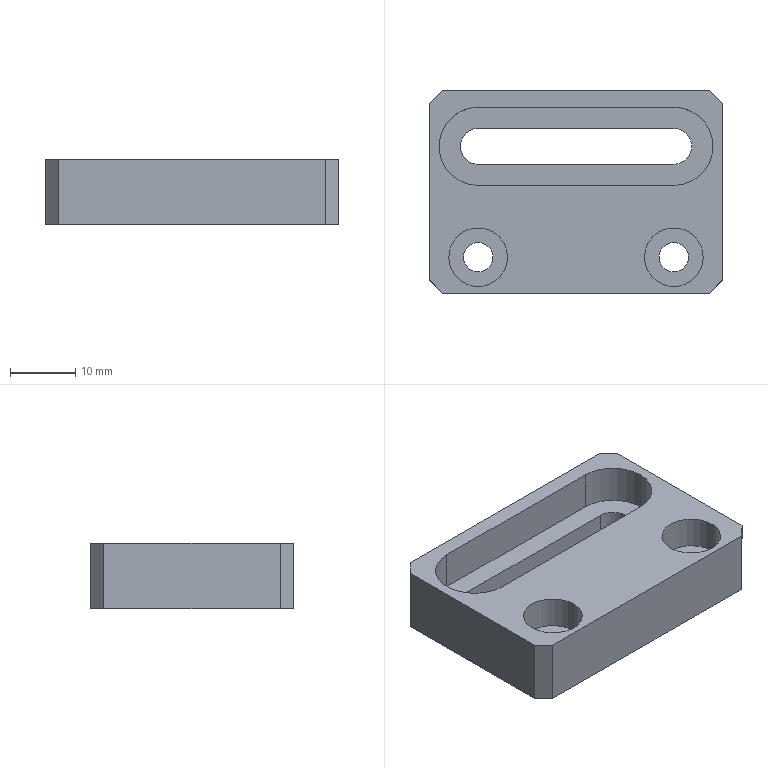Part | SolidWorks | features ICE 4, Chamfer 1, Extrusion 1 | 1 solid | 31 faces | box 45 x 31 x 10 mm | volume 9481 mm3 | plane 17 | cylinder 14 | commonest cylinder face diameters 4.5 x4 9 x4 5.5 x3 12 x3
STEP:
#1=CARTESIAN_POINT('',(21.,7.,4.));
#2=VERTEX_POINT('',#1);
#3=CARTESIAN_POINT('',(15.,13.,4.));
#4=VERTEX_POINT('',#3);
#5=CARTESIAN_POINT('',(15.,7.,4.));
#6=DIRECTION('',(0.,0.,1.));
#7=DIRECTION('',(1.,0.,0.));
#8=AXIS2_PLACEMENT_3D('',#5,#6,#7);
#9=CIRCLE('',#8,6.);
#10=EDGE_CURVE('',#2,#4,#9,.T.);
#11=ORIENTED_EDGE('',*,*,#10,.F.);
#12=CARTESIAN_POINT('',(21.,7.,10.));
#13=VERTEX_POINT('',#12);
#14=CARTESIAN_POINT('',(21.,7.,4.));
#15=DIRECTION('',(0.,0.,1.));
#16=VECTOR('',#15,1000.);
#17=LINE('',#14,#16);
#18=EDGE_CURVE('',#2,#13,#17,.T.);
#19=ORIENTED_EDGE('',*,*,#18,.T.);
#20=CARTESIAN_POINT('',(15.,13.,10.));
#21=VERTEX_POINT('',#20);
#22=CARTESIAN_POINT('',(15.,7.,10.));
#23=DIRECTION('',(0.,0.,1.));
#24=DIRECTION('',(1.,0.,0.));
#25=AXIS2_PLACEMENT_3D('',#22,#23,#24);
#26=CIRCLE('',#25,6.);
#27=EDGE_CURVE('',#13,#21,#26,.T.);
#28=ORIENTED_EDGE('',*,*,#27,.T.);
#29=CARTESIAN_POINT('',(15.,13.,4.));
#30=DIRECTION('',(0.,0.,1.));
#31=VECTOR('',#30,1000.);
#32=LINE('',#29,#31);
#33=EDGE_CURVE('',#4,#21,#32,.T.);
#34=ORIENTED_EDGE('',*,*,#33,.F.);
#35=EDGE_LOOP('',(#11,#19,#28,#34));
#36=FACE_OUTER_BOUND('',#35,.T.);
#37=CARTESIAN_POINT('',(15.,7.,4.));
#38=DIRECTION('',(0.,0.,1.));
#39=DIRECTION('',(1.,0.,0.));
#40=AXIS2_PLACEMENT_3D('',#37,#38,#39);
#41=CYLINDRICAL_SURFACE('',#40,6.);
#42=ADVANCED_FACE('',(#36),#41,.F.);
#43=CARTESIAN_POINT('',(12.75,-10.,0.));
#44=VERTEX_POINT('',#43);
#45=CARTESIAN_POINT('',(17.25,-10.,0.));
#46=VERTEX_POINT('',#45);
#47=CARTESIAN_POINT('',(15.,-10.,0.));
#48=DIRECTION('',(0.,0.,1.));
#49=DIRECTION('',(1.,0.,0.));
#50=AXIS2_PLACEMENT_3D('',#47,#48,#49);
#51=CIRCLE('',#50,2.25);
#52=EDGE_CURVE('',#44,#46,#51,.T.);
#53=ORIENTED_EDGE('',*,*,#52,.F.);
#54=CARTESIAN_POINT('',(12.75,-10.,5.));
#55=VERTEX_POINT('',#54);
#56=CARTESIAN_POINT('',(12.75,-10.,-4.));
#57=DIRECTION('',(0.,0.,1.));
#58=VECTOR('',#57,1000.);
#59=LINE('',#56,#58);
#60=EDGE_CURVE('',#44,#55,#59,.T.);
#61=ORIENTED_EDGE('',*,*,#60,.T.);
#62=CARTESIAN_POINT('',(17.25,-10.,5.));
#63=VERTEX_POINT('',#62);
#64=CARTESIAN_POINT('',(15.,-10.,5.));
#65=DIRECTION('',(0.,0.,-1.));
#66=DIRECTION('',(-1.,0.,0.));
#67=AXIS2_PLACEMENT_3D('',#64,#65,#66);
#68=CIRCLE('',#67,2.25);
#69=EDGE_CURVE('',#63,#55,#68,.T.);
#70=ORIENTED_EDGE('',*,*,#69,.F.);
#71=CARTESIAN_POINT('',(17.25,-10.,-4.));
#72=DIRECTION('',(0.,0.,1.));
#73=VECTOR('',#72,1000.);
#74=LINE('',#71,#73);
#75=EDGE_CURVE('',#46,#63,#74,.T.);
#76=ORIENTED_EDGE('',*,*,#75,.F.);
#77=EDGE_LOOP('',(#53,#61,#70,#76));
#78=FACE_OUTER_BOUND('',#77,.T.);
#79=CARTESIAN_POINT('',(15.,-10.,-4.));
#80=DIRECTION('',(0.,0.,1.));
#81=DIRECTION('',(1.,0.,0.));
#82=AXIS2_PLACEMENT_3D('',#79,#80,#81);
#83=CYLINDRICAL_SURFACE('',#82,2.25);
#84=ADVANCED_FACE('',(#78),#83,.F.);
#85=CARTESIAN_POINT('',(-17.25,-10.,0.));
#86=VERTEX_POINT('',#85);
#87=CARTESIAN_POINT('',(-12.75,-10.,0.));
#88=VERTEX_POINT('',#87);
#89=CARTESIAN_POINT('',(-15.,-10.,0.));
#90=DIRECTION('',(0.,0.,1.));
#91=DIRECTION('',(1.,0.,0.));
#92=AXIS2_PLACEMENT_3D('',#89,#90,#91);
#93=CIRCLE('',#92,2.25);
#94=EDGE_CURVE('',#86,#88,#93,.T.);
#95=ORIENTED_EDGE('',*,*,#94,.F.);
#96=CARTESIAN_POINT('',(-17.25,-10.,5.));
#97=VERTEX_POINT('',#96);
#98=CARTESIAN_POINT('',(-17.25,-10.,-4.));
#99=DIRECTION('',(0.,0.,1.));
#100=VECTOR('',#99,1000.);
#101=LINE('',#98,#100);
#102=EDGE_CURVE('',#86,#97,#101,.T.);
#103=ORIENTED_EDGE('',*,*,#102,.T.);
#104=CARTESIAN_POINT('',(-12.75,-10.,5.));
#105=VERTEX_POINT('',#104);
#106=CARTESIAN_POINT('',(-15.,-10.,5.));
#107=DIRECTION('',(0.,0.,1.));
#108=DIRECTION('',(1.,0.,0.));
#109=AXIS2_PLACEMENT_3D('',#106,#107,#108);
#110=CIRCLE('',#109,2.25);
#111=EDGE_CURVE('',#97,#105,#110,.T.);
#112=ORIENTED_EDGE('',*,*,#111,.T.);
#113=CARTESIAN_POINT('',(-12.75,-10.,-4.));
#114=DIRECTION('',(0.,0.,1.));
#115=VECTOR('',#114,1000.);
#116=LINE('',#113,#115);
#117=EDGE_CURVE('',#88,#105,#116,.T.);
#118=ORIENTED_EDGE('',*,*,#117,.F.);
#119=EDGE_LOOP('',(#95,#103,#112,#118));
#120=FACE_OUTER_BOUND('',#119,.T.);
#121=CARTESIAN_POINT('',(-15.,-10.,-4.));
#122=DIRECTION('',(0.,0.,1.));
#123=DIRECTION('',(1.,0.,0.));
#124=AXIS2_PLACEMENT_3D('',#121,#122,#123);
#125=CYLINDRICAL_SURFACE('',#124,2.25);
#126=ADVANCED_FACE('',(#120),#125,.F.);
#127=CARTESIAN_POINT('',(10.5,-10.,5.));
#128=VERTEX_POINT('',#127);
#129=CARTESIAN_POINT('',(19.5,-10.,5.));
#130=VERTEX_POINT('',#129);
#131=CARTESIAN_POINT('',(15.,-10.,5.));
#132=DIRECTION('',(0.,0.,1.));
#133=DIRECTION('',(-1.,0.,0.));
#134=AXIS2_PLACEMENT_3D('',#131,#132,#133);
#135=CIRCLE('',#134,4.5);
#136=EDGE_CURVE('',#128,#130,#135,.T.);
#137=ORIENTED_EDGE('',*,*,#136,.F.);
#138=CARTESIAN_POINT('',(10.5,-10.,10.));
#139=VERTEX_POINT('',#138);
#140=CARTESIAN_POINT('',(10.5,-10.,5.));
#141=DIRECTION('',(0.,0.,1.));
#142=VECTOR('',#141,1000.);
#143=LINE('',#140,#142);
#144=EDGE_CURVE('',#128,#139,#143,.T.);
#145=ORIENTED_EDGE('',*,*,#144,.T.);
#146=CARTESIAN_POINT('',(19.5,-10.,10.));
#147=VERTEX_POINT('',#146);
#148=CARTESIAN_POINT('',(15.,-10.,10.));
#149=DIRECTION('',(0.,0.,1.));
#150=DIRECTION('',(-1.,0.,0.));
#151=AXIS2_PLACEMENT_3D('',#148,#149,#150);
#152=CIRCLE('',#151,4.5);
#153=EDGE_CURVE('',#139,#147,#152,.T.);
#154=ORIENTED_EDGE('',*,*,#153,.T.);
#155=CARTESIAN_POINT('',(19.5,-10.,5.));
#156=DIRECTION('',(0.,0.,1.));
#157=VECTOR('',#156,1000.);
#158=LINE('',#155,#157);
#159=EDGE_CURVE('',#130,#147,#158,.T.);
#160=ORIENTED_EDGE('',*,*,#159,.F.);
#161=EDGE_LOOP('',(#137,#145,#154,#160));
#162=FACE_OUTER_BOUND('',#161,.T.);
#163=CARTESIAN_POINT('',(15.,-10.,5.));
#164=DIRECTION('',(0.,0.,1.));
#165=DIRECTION('',(1.,0.,0.));
#166=AXIS2_PLACEMENT_3D('',#163,#164,#165);
#167=CYLINDRICAL_SURFACE('',#166,4.5);
#168=ADVANCED_FACE('',(#162),#167,.F.);
#169=CARTESIAN_POINT('',(-19.5,-10.,5.));
#170=VERTEX_POINT('',#169);
#171=CARTESIAN_POINT('',(-10.5,-10.,5.));
#172=VERTEX_POINT('',#171);
#173=CARTESIAN_POINT('',(-15.,-10.,5.));
#174=DIRECTION('',(0.,0.,1.));
#175=DIRECTION('',(1.,0.,0.));
#176=AXIS2_PLACEMENT_3D('',#173,#174,#175);
#177=CIRCLE('',#176,4.5);
#178=EDGE_CURVE('',#170,#172,#177,.T.);
#179=ORIENTED_EDGE('',*,*,#178,.F.);
#180=CARTESIAN_POINT('',(-19.5,-10.,10.));
#181=VERTEX_POINT('',#180);
#182=CARTESIAN_POINT('',(-19.5,-10.,5.));
#183=DIRECTION('',(0.,0.,1.));
#184=VECTOR('',#183,1000.);
#185=LINE('',#182,#184);
#186=EDGE_CURVE('',#170,#181,#185,.T.);
#187=ORIENTED_EDGE('',*,*,#186,.T.);
#188=CARTESIAN_POINT('',(-10.5,-10.,10.));
#189=VERTEX_POINT('',#188);
#190=CARTESIAN_POINT('',(-15.,-10.,10.));
#191=DIRECTION('',(0.,0.,1.));
#192=DIRECTION('',(1.,0.,0.));
#193=AXIS2_PLACEMENT_3D('',#190,#191,#192);
#194=CIRCLE('',#193,4.5);
#195=EDGE_CURVE('',#181,#189,#194,.T.);
#196=ORIENTED_EDGE('',*,*,#195,.T.);
#197=CARTESIAN_POINT('',(-10.5,-10.,5.));
#198=DIRECTION('',(0.,0.,1.));
#199=VECTOR('',#198,1000.);
#200=LINE('',#197,#199);
#201=EDGE_CURVE('',#172,#189,#200,.T.);
#202=ORIENTED_EDGE('',*,*,#201,.F.);
#203=EDGE_LOOP('',(#179,#187,#196,#202));
#204=FACE_OUTER_BOUND('',#203,.T.);
#205=CARTESIAN_POINT('',(-15.,-10.,5.));
#206=DIRECTION('',(0.,0.,1.));
#207=DIRECTION('',(1.,0.,0.));
#208=AXIS2_PLACEMENT_3D('',#205,#206,#207);
#209=CYLINDRICAL_SURFACE('',#208,4.5);
#210=ADVANCED_FACE('',(#204),#209,.F.);
#211=CARTESIAN_POINT('',(17.75,7.,0.));
#212=VERTEX_POINT('',#211);
#213=CARTESIAN_POINT('',(15.,9.75,0.));
#214=VERTEX_POINT('',#213);
#215=CARTESIAN_POINT('',(15.,7.,0.));
#216=DIRECTION('',(0.,0.,1.));
#217=DIRECTION('',(1.,0.,0.));
#218=AXIS2_PLACEMENT_3D('',#215,#216,#217);
#219=CIRCLE('',#218,2.75);
#220=EDGE_CURVE('',#212,#214,#219,.T.);
#221=ORIENTED_EDGE('',*,*,#220,.F.);
#222=CARTESIAN_POINT('',(17.75,7.,4.));
#223=VERTEX_POINT('',#222);
#224=CARTESIAN_POINT('',(17.75,7.,-3.));
#225=DIRECTION('',(0.,0.,1.));
#226=VECTOR('',#225,1000.);
#227=LINE('',#224,#226);
#228=EDGE_CURVE('',#212,#223,#227,.T.);
#229=ORIENTED_EDGE('',*,*,#228,.T.);
#230=CARTESIAN_POINT('',(15.,9.75,4.));
#231=VERTEX_POINT('',#230);
#232=CARTESIAN_POINT('',(15.,7.,4.));
#233=DIRECTION('',(0.,0.,-1.));
#234=DIRECTION('',(1.,0.,0.));
#235=AXIS2_PLACEMENT_3D('',#232,#233,#234);
#236=CIRCLE('',#235,2.75);
#237=EDGE_CURVE('',#231,#223,#236,.T.);
#238=ORIENTED_EDGE('',*,*,#237,.F.);
#239=CARTESIAN_POINT('',(15.,9.75,-3.));
#240=DIRECTION('',(0.,0.,1.));
#241=VECTOR('',#240,1000.);
#242=LINE('',#239,#241);
#243=EDGE_CURVE('',#214,#231,#242,.T.);
#244=ORIENTED_EDGE('',*,*,#243,.F.);
#245=EDGE_LOOP('',(#221,#229,#238,#244));
#246=FACE_OUTER_BOUND('',#245,.T.);
#247=CARTESIAN_POINT('',(15.,7.,-3.));
#248=DIRECTION('',(0.,0.,1.));
#249=DIRECTION('',(1.,0.,0.));
#250=AXIS2_PLACEMENT_3D('',#247,#248,#249);
#251=CYLINDRICAL_SURFACE('',#250,2.75);
#252=ADVANCED_FACE('',(#246),#251,.F.);
#253=CARTESIAN_POINT('',(-15.,4.25,4.));
#254=VERTEX_POINT('',#253);
#255=CARTESIAN_POINT('',(-15.,9.75,4.));
#256=VERTEX_POINT('',#255);
#257=CARTESIAN_POINT('',(-15.,7.,4.));
#258=DIRECTION('',(0.,0.,-1.));
#259=DIRECTION('',(1.,0.,0.));
#260=AXIS2_PLACEMENT_3D('',#257,#258,#259);
#261=CIRCLE('',#260,2.75);
#262=EDGE_CURVE('',#254,#256,#261,.T.);
#263=ORIENTED_EDGE('',*,*,#262,.F.);
#264=CARTESIAN_POINT('',(-15.,4.25,0.));
#265=VERTEX_POINT('',#264);
#266=CARTESIAN_POINT('',(-15.,4.25,-3.));
#267=DIRECTION('',(0.,0.,1.));
#268=VECTOR('',#267,1000.);
#269=LINE('',#266,#268);
#270=EDGE_CURVE('',#265,#254,#269,.T.);
#271=ORIENTED_EDGE('',*,*,#270,.F.);
#272=CARTESIAN_POINT('',(-15.,9.75,0.));
#273=VERTEX_POINT('',#272);
#274=CARTESIAN_POINT('',(-15.,7.,0.));
#275=DIRECTION('',(0.,0.,1.));
#276=DIRECTION('',(1.,0.,0.));
#277=AXIS2_PLACEMENT_3D('',#274,#275,#276);
#278=CIRCLE('',#277,2.75);
#279=EDGE_CURVE('',#273,#265,#278,.T.);
#280=ORIENTED_EDGE('',*,*,#279,.F.);
#281=CARTESIAN_POINT('',(-15.,9.75,-3.));
#282=DIRECTION('',(0.,0.,1.));
#283=VECTOR('',#282,1000.);
#284=LINE('',#281,#283);
#285=EDGE_CURVE('',#273,#256,#284,.T.);
#286=ORIENTED_EDGE('',*,*,#285,.T.);
#287=EDGE_LOOP('',(#263,#271,#280,#286));
#288=FACE_OUTER_BOUND('',#287,.T.);
#289=CARTESIAN_POINT('',(-15.,7.,-3.));
#290=DIRECTION('',(0.,0.,1.));
#291=DIRECTION('',(1.,0.,0.));
#292=AXIS2_PLACEMENT_3D('',#289,#290,#291);
#293=CYLINDRICAL_SURFACE('',#292,2.75);
#294=ADVANCED_FACE('',(#288),#293,.F.);
#295=CARTESIAN_POINT('',(-15.,9.75,4.));
#296=DIRECTION('',(1.,0.,0.));
#297=VECTOR('',#296,1000.);
#298=LINE('',#295,#297);
#299=EDGE_CURVE('',#256,#231,#298,.T.);
#300=ORIENTED_EDGE('',*,*,#299,.F.);
#301=ORIENTED_EDGE('',*,*,#285,.F.);
#302=CARTESIAN_POINT('',(0.,9.75,0.));
#303=DIRECTION('',(-1.,0.,0.));
#304=VECTOR('',#303,1000.);
#305=LINE('',#302,#304);
#306=EDGE_CURVE('',#214,#273,#305,.T.);
#307=ORIENTED_EDGE('',*,*,#306,.F.);
#308=ORIENTED_EDGE('',*,*,#243,.T.);
#309=EDGE_LOOP('',(#300,#301,#307,#308));
#310=FACE_OUTER_BOUND('',#309,.T.);
#311=CARTESIAN_POINT('',(-15.,9.75,-3.));
#312=DIRECTION('',(0.,1.,0.));
#313=DIRECTION('',(-1.,0.,0.));
#314=AXIS2_PLACEMENT_3D('',#311,#312,#313);
#315=PLANE('',#314);
#316=ADVANCED_FACE('',(#310),#315,.F.);
#317=ORIENTED_EDGE('',*,*,#228,.F.);
#318=CARTESIAN_POINT('',(15.,4.25,0.));
#319=VERTEX_POINT('',#318);
#320=CARTESIAN_POINT('',(15.,7.,0.));
#321=DIRECTION('',(0.,0.,1.));
#322=DIRECTION('',(1.,0.,0.));
#323=AXIS2_PLACEMENT_3D('',#320,#321,#322);
#324=CIRCLE('',#323,2.75);
#325=EDGE_CURVE('',#319,#212,#324,.T.);
#326=ORIENTED_EDGE('',*,*,#325,.F.);
#327=CARTESIAN_POINT('',(15.,4.25,4.));
#328=VERTEX_POINT('',#327);
#329=CARTESIAN_POINT('',(15.,4.25,-3.));
#330=DIRECTION('',(0.,0.,1.));
#331=VECTOR('',#330,1000.);
#332=LINE('',#329,#331);
#333=EDGE_CURVE('',#319,#328,#332,.T.);
#334=ORIENTED_EDGE('',*,*,#333,.T.);
#335=CARTESIAN_POINT('',(15.,7.,4.));
#336=DIRECTION('',(0.,0.,-1.));
#337=DIRECTION('',(1.,0.,0.));
#338=AXIS2_PLACEMENT_3D('',#335,#336,#337);
#339=CIRCLE('',#338,2.75);
#340=EDGE_CURVE('',#223,#328,#339,.T.);
#341=ORIENTED_EDGE('',*,*,#340,.F.);
#342=EDGE_LOOP('',(#317,#326,#334,#341));
#343=FACE_OUTER_BOUND('',#342,.T.);
#344=CARTESIAN_POINT('',(15.,7.,-3.));
#345=DIRECTION('',(0.,0.,1.));
#346=DIRECTION('',(1.,0.,0.));
#347=AXIS2_PLACEMENT_3D('',#344,#345,#346);
#348=CYLINDRICAL_SURFACE('',#347,2.75);
#349=ADVANCED_FACE('',(#343),#348,.F.);
#350=CARTESIAN_POINT('',(-15.,4.25,4.));
#351=DIRECTION('',(-1.,0.,0.));
#352=VECTOR('',#351,1000.);
#353=LINE('',#350,#352);
#354=EDGE_CURVE('',#328,#254,#353,.T.);
#355=ORIENTED_EDGE('',*,*,#354,.F.);
#356=ORIENTED_EDGE('',*,*,#333,.F.);
#357=CARTESIAN_POINT('',(0.,4.25,0.));
#358=DIRECTION('',(1.,0.,0.));
#359=VECTOR('',#358,1000.);
#360=LINE('',#357,#359);
#361=EDGE_CURVE('',#265,#319,#360,.T.);
#362=ORIENTED_EDGE('',*,*,#361,.F.);
#363=ORIENTED_EDGE('',*,*,#270,.T.);
#364=EDGE_LOOP('',(#355,#356,#362,#363));
#365=FACE_OUTER_BOUND('',#364,.T.);
#366=CARTESIAN_POINT('',(-15.,4.25,-3.));
#367=DIRECTION('',(0.,-1.,0.));
#368=DIRECTION('',(0.,0.,-1.));
#369=AXIS2_PLACEMENT_3D('',#366,#367,#368);
#370=PLANE('',#369);
#371=ADVANCED_FACE('',(#365),#370,.F.);
#372=CARTESIAN_POINT('',(22.5,-13.5,0.));
#373=VERTEX_POINT('',#372);
#374=CARTESIAN_POINT('',(22.5,13.5,0.));
#375=VERTEX_POINT('',#374);
#376=CARTESIAN_POINT('',(22.5,15.5,0.));
#377=DIRECTION('',(0.,1.,0.));
#378=VECTOR('',#377,1000.);
#379=LINE('',#376,#378);
#380=EDGE_CURVE('',#373,#375,#379,.T.);
#381=ORIENTED_EDGE('',*,*,#380,.T.);
#382=CARTESIAN_POINT('',(22.5,13.5,10.));
#383=VERTEX_POINT('',#382);
#384=CARTESIAN_POINT('',(22.5,13.5,10.));
#385=DIRECTION('',(0.,0.,1.));
#386=VECTOR('',#385,1000.);
#387=LINE('',#384,#386);
#388=EDGE_CURVE('',#375,#383,#387,.T.);
#389=ORIENTED_EDGE('',*,*,#388,.T.);
#390=CARTESIAN_POINT('',(22.5,-13.5,10.));
#391=VERTEX_POINT('',#390);
#392=CARTESIAN_POINT('',(22.5,15.5,10.));
#393=DIRECTION('',(0.,1.,0.));
#394=VECTOR('',#393,1000.);
#395=LINE('',#392,#394);
#396=EDGE_CURVE('',#391,#383,#395,.T.);
#397=ORIENTED_EDGE('',*,*,#396,.F.);
#398=CARTESIAN_POINT('',(22.5,-13.5,10.));
#399=DIRECTION('',(0.,0.,-1.));
#400=VECTOR('',#399,1000.);
#401=LINE('',#398,#400);
#402=EDGE_CURVE('',#391,#373,#401,.T.);
#403=ORIENTED_EDGE('',*,*,#402,.T.);
#404=EDGE_LOOP('',(#381,#389,#397,#403));
#405=FACE_OUTER_BOUND('',#404,.T.);
#406=CARTESIAN_POINT('',(22.5,15.5,10.));
#407=DIRECTION('',(-1.,0.,0.));
#408=DIRECTION('',(0.,-1.,0.));
#409=AXIS2_PLACEMENT_3D('',#406,#407,#408);
#410=PLANE('',#409);
#411=ADVANCED_FACE('',(#405),#410,.F.);
#412=CARTESIAN_POINT('',(20.5,15.5,10.));
#413=VERTEX_POINT('',#412);
#414=CARTESIAN_POINT('',(-20.5,15.5,10.));
#415=VERTEX_POINT('',#414);
#416=CARTESIAN_POINT('',(-22.5,15.5,10.));
#417=DIRECTION('',(-1.,0.,0.));
#418=VECTOR('',#417,1000.);
#419=LINE('',#416,#418);
#420=EDGE_CURVE('',#413,#415,#419,.T.);
#421=ORIENTED_EDGE('',*,*,#420,.F.);
#422=CARTESIAN_POINT('',(20.5,15.5,0.));
#423=VERTEX_POINT('',#422);
#424=CARTESIAN_POINT('',(20.5,15.5,10.));
#425=DIRECTION('',(0.,0.,-1.));
#426=VECTOR('',#425,1000.);
#427=LINE('',#424,#426);
#428=EDGE_CURVE('',#413,#423,#427,.T.);
#429=ORIENTED_EDGE('',*,*,#428,.T.);
#430=CARTESIAN_POINT('',(-20.5,15.5,0.));
#431=VERTEX_POINT('',#430);
#432=CARTESIAN_POINT('',(-22.5,15.5,0.));
#433=DIRECTION('',(-1.,0.,0.));
#434=VECTOR('',#433,1000.);
#435=LINE('',#432,#434);
#436=EDGE_CURVE('',#423,#431,#435,.T.);
#437=ORIENTED_EDGE('',*,*,#436,.T.);
#438=CARTESIAN_POINT('',(-20.5,15.5,10.));
#439=DIRECTION('',(0.,0.,1.));
#440=VECTOR('',#439,1000.);
#441=LINE('',#438,#440);
#442=EDGE_CURVE('',#431,#415,#441,.T.);
#443=ORIENTED_EDGE('',*,*,#442,.T.);
#444=EDGE_LOOP('',(#421,#429,#437,#443));
#445=FACE_OUTER_BOUND('',#444,.T.);
#446=CARTESIAN_POINT('',(-22.5,15.5,10.));
#447=DIRECTION('',(0.,-1.,0.));
#448=DIRECTION('',(0.,0.,-1.));
#449=AXIS2_PLACEMENT_3D('',#446,#447,#448);
#450=PLANE('',#449);
#451=ADVANCED_FACE('',(#445),#450,.F.);
#452=CARTESIAN_POINT('',(-22.5,13.5,0.));
#453=VERTEX_POINT('',#452);
#454=CARTESIAN_POINT('',(-22.5,-13.5,0.));
#455=VERTEX_POINT('',#454);
#456=CARTESIAN_POINT('',(-22.5,15.5,0.));
#457=DIRECTION('',(0.,-1.,0.));
#458=VECTOR('',#457,1000.);
#459=LINE('',#456,#458);
#460=EDGE_CURVE('',#453,#455,#459,.T.);
#461=ORIENTED_EDGE('',*,*,#460,.T.);
#462=CARTESIAN_POINT('',(-22.5,-13.5,10.));
#463=VERTEX_POINT('',#462);
#464=CARTESIAN_POINT('',(-22.5,-13.5,10.));
#465=DIRECTION('',(0.,0.,1.));
#466=VECTOR('',#465,1000.);
#467=LINE('',#464,#466);
#468=EDGE_CURVE('',#455,#463,#467,.T.);
#469=ORIENTED_EDGE('',*,*,#468,.T.);
#470=CARTESIAN_POINT('',(-22.5,13.5,10.));
#471=VERTEX_POINT('',#470);
#472=CARTESIAN_POINT('',(-22.5,15.5,10.));
#473=DIRECTION('',(0.,-1.,0.));
#474=VECTOR('',#473,1000.);
#475=LINE('',#472,#474);
#476=EDGE_CURVE('',#471,#463,#475,.T.);
#477=ORIENTED_EDGE('',*,*,#476,.F.);
#478=CARTESIAN_POINT('',(-22.5,13.5,10.));
#479=DIRECTION('',(0.,0.,-1.));
#480=VECTOR('',#479,1000.);
#481=LINE('',#478,#480);
#482=EDGE_CURVE('',#471,#453,#481,.T.);
#483=ORIENTED_EDGE('',*,*,#482,.T.);
#484=EDGE_LOOP('',(#461,#469,#477,#483));
#485=FACE_OUTER_BOUND('',#484,.T.);
#486=CARTESIAN_POINT('',(-22.5,15.5,10.));
#487=DIRECTION('',(1.,0.,0.));
#488=DIRECTION('',(0.,1.,0.));
#489=AXIS2_PLACEMENT_3D('',#486,#487,#488);
#490=PLANE('',#489);
#491=ADVANCED_FACE('',(#485),#490,.F.);
#492=CARTESIAN_POINT('',(-20.5,-15.5,0.));
#493=VERTEX_POINT('',#492);
#494=CARTESIAN_POINT('',(20.5,-15.5,0.));
#495=VERTEX_POINT('',#494);
#496=CARTESIAN_POINT('',(-22.5,-15.5,0.));
#497=DIRECTION('',(1.,0.,0.));
#498=VECTOR('',#497,1000.);
#499=LINE('',#496,#498);
#500=EDGE_CURVE('',#493,#495,#499,.T.);
#501=ORIENTED_EDGE('',*,*,#500,.T.);
#502=CARTESIAN_POINT('',(20.5,-15.5,10.));
#503=VERTEX_POINT('',#502);
#504=CARTESIAN_POINT('',(20.5,-15.5,10.));
#505=DIRECTION('',(0.,0.,1.));
#506=VECTOR('',#505,1000.);
#507=LINE('',#504,#506);
#508=EDGE_CURVE('',#495,#503,#507,.T.);
#509=ORIENTED_EDGE('',*,*,#508,.T.);
#510=CARTESIAN_POINT('',(-20.5,-15.5,10.));
#511=VERTEX_POINT('',#510);
#512=CARTESIAN_POINT('',(-22.5,-15.5,10.));
#513=DIRECTION('',(1.,0.,0.));
#514=VECTOR('',#513,1000.);
#515=LINE('',#512,#514);
#516=EDGE_CURVE('',#511,#503,#515,.T.);
#517=ORIENTED_EDGE('',*,*,#516,.F.);
#518=CARTESIAN_POINT('',(-20.5,-15.5,10.));
#519=DIRECTION('',(0.,0.,-1.));
#520=VECTOR('',#519,1000.);
#521=LINE('',#518,#520);
#522=EDGE_CURVE('',#511,#493,#521,.T.);
#523=ORIENTED_EDGE('',*,*,#522,.T.);
#524=EDGE_LOOP('',(#501,#509,#517,#523));
#525=FACE_OUTER_BOUND('',#524,.T.);
#526=CARTESIAN_POINT('',(-22.5,-15.5,10.));
#527=DIRECTION('',(0.,1.,0.));
#528=DIRECTION('',(0.,0.,1.));
#529=AXIS2_PLACEMENT_3D('',#526,#527,#528);
#530=PLANE('',#529);
#531=ADVANCED_FACE('',(#525),#530,.F.);
#532=CARTESIAN_POINT('',(-15.,13.,10.));
#533=VERTEX_POINT('',#532);
#534=CARTESIAN_POINT('',(-15.,1.,10.));
#535=VERTEX_POINT('',#534);
#536=CARTESIAN_POINT('',(-15.,7.,10.));
#537=DIRECTION('',(0.,0.,1.));
#538=DIRECTION('',(1.,0.,0.));
#539=AXIS2_PLACEMENT_3D('',#536,#537,#538);
#540=CIRCLE('',#539,6.);
#541=EDGE_CURVE('',#533,#535,#540,.T.);
#542=ORIENTED_EDGE('',*,*,#541,.F.);
#543=CARTESIAN_POINT('',(-15.,13.,10.));
#544=DIRECTION('',(-1.,0.,0.));
#545=VECTOR('',#544,1000.);
#546=LINE('',#543,#545);
#547=EDGE_CURVE('',#21,#533,#546,.T.);
#548=ORIENTED_EDGE('',*,*,#547,.F.);
#549=ORIENTED_EDGE('',*,*,#27,.F.);
#550=CARTESIAN_POINT('',(15.,1.,10.));
#551=VERTEX_POINT('',#550);
#552=CARTESIAN_POINT('',(15.,7.,10.));
#553=DIRECTION('',(0.,0.,1.));
#554=DIRECTION('',(1.,0.,0.));
#555=AXIS2_PLACEMENT_3D('',#552,#553,#554);
#556=CIRCLE('',#555,6.);
#557=EDGE_CURVE('',#551,#13,#556,.T.);
#558=ORIENTED_EDGE('',*,*,#557,.F.);
#559=CARTESIAN_POINT('',(-15.,1.,10.));
#560=DIRECTION('',(1.,0.,0.));
#561=VECTOR('',#560,1000.);
#562=LINE('',#559,#561);
#563=EDGE_CURVE('',#535,#551,#562,.T.);
#564=ORIENTED_EDGE('',*,*,#563,.F.);
#565=EDGE_LOOP('',(#542,#548,#549,#558,#564));
#566=FACE_BOUND('',#565,.T.);
#567=CARTESIAN_POINT('',(15.,-10.,10.));
#568=DIRECTION('',(0.,0.,1.));
#569=DIRECTION('',(-1.,0.,0.));
#570=AXIS2_PLACEMENT_3D('',#567,#568,#569);
#571=CIRCLE('',#570,4.5);
#572=EDGE_CURVE('',#147,#139,#571,.T.);
#573=ORIENTED_EDGE('',*,*,#572,.F.);
#574=ORIENTED_EDGE('',*,*,#153,.F.);
#575=EDGE_LOOP('',(#573,#574));
#576=FACE_BOUND('',#575,.T.);
#577=CARTESIAN_POINT('',(-15.,-10.,10.));
#578=DIRECTION('',(0.,0.,1.));
#579=DIRECTION('',(1.,0.,0.));
#580=AXIS2_PLACEMENT_3D('',#577,#578,#579);
#581=CIRCLE('',#580,4.5);
#582=EDGE_CURVE('',#189,#181,#581,.T.);
#583=ORIENTED_EDGE('',*,*,#582,.F.);
#584=ORIENTED_EDGE('',*,*,#195,.F.);
#585=EDGE_LOOP('',(#583,#584));
#586=FACE_BOUND('',#585,.T.);
#587=ORIENTED_EDGE('',*,*,#396,.T.);
#588=CARTESIAN_POINT('',(18.,18.,10.));
#589=DIRECTION('',(-0.7071,0.7071,0.));
#590=VECTOR('',#589,1000.);
#591=LINE('',#588,#590);
#592=EDGE_CURVE('',#383,#413,#591,.T.);
#593=ORIENTED_EDGE('',*,*,#592,.T.);
#594=ORIENTED_EDGE('',*,*,#420,.T.);
#595=CARTESIAN_POINT('',(-18.,18.,10.));
#596=DIRECTION('',(-0.7071,-0.7071,0.));
#597=VECTOR('',#596,1000.);
#598=LINE('',#595,#597);
#599=EDGE_CURVE('',#415,#471,#598,.T.);
#600=ORIENTED_EDGE('',*,*,#599,.T.);
#601=ORIENTED_EDGE('',*,*,#476,.T.);
#602=CARTESIAN_POINT('',(-18.,-18.,10.));
#603=DIRECTION('',(0.7071,-0.7071,0.));
#604=VECTOR('',#603,1000.);
#605=LINE('',#602,#604);
#606=EDGE_CURVE('',#463,#511,#605,.T.);
#607=ORIENTED_EDGE('',*,*,#606,.T.);
#608=ORIENTED_EDGE('',*,*,#516,.T.);
#609=CARTESIAN_POINT('',(18.,-18.,10.));
#610=DIRECTION('',(0.7071,0.7071,0.));
#611=VECTOR('',#610,1000.);
#612=LINE('',#609,#611);
#613=EDGE_CURVE('',#503,#391,#612,.T.);
#614=ORIENTED_EDGE('',*,*,#613,.T.);
#615=EDGE_LOOP('',(#587,#593,#594,#600,#601,#607,#608,#614));
#616=FACE_OUTER_BOUND('',#615,.T.);
#617=CARTESIAN_POINT('',(0.,0.,10.));
#618=DIRECTION('',(0.,0.,1.));
#619=DIRECTION('',(1.,0.,0.));
#620=AXIS2_PLACEMENT_3D('',#617,#618,#619);
#621=PLANE('',#620);
#622=ADVANCED_FACE('',(#566,#576,#586,#616),#621,.T.);
#623=CARTESIAN_POINT('',(15.,-10.,0.));
#624=DIRECTION('',(0.,0.,1.));
#625=DIRECTION('',(1.,0.,0.));
#626=AXIS2_PLACEMENT_3D('',#623,#624,#625);
#627=CIRCLE('',#626,2.25);
#628=EDGE_CURVE('',#46,#44,#627,.T.);
#629=ORIENTED_EDGE('',*,*,#628,.T.);
#630=ORIENTED_EDGE('',*,*,#52,.T.);
#631=EDGE_LOOP('',(#629,#630));
#632=FACE_BOUND('',#631,.T.);
#633=CARTESIAN_POINT('',(-15.,-10.,0.));
#634=DIRECTION('',(0.,0.,1.));
#635=DIRECTION('',(1.,0.,0.));
#636=AXIS2_PLACEMENT_3D('',#633,#634,#635);
#637=CIRCLE('',#636,2.25);
#638=EDGE_CURVE('',#88,#86,#637,.T.);
#639=ORIENTED_EDGE('',*,*,#638,.T.);
#640=ORIENTED_EDGE('',*,*,#94,.T.);
#641=EDGE_LOOP('',(#639,#640));
#642=FACE_BOUND('',#641,.T.);
#643=ORIENTED_EDGE('',*,*,#306,.T.);
#644=ORIENTED_EDGE('',*,*,#279,.T.);
#645=ORIENTED_EDGE('',*,*,#361,.T.);
#646=ORIENTED_EDGE('',*,*,#325,.T.);
#647=ORIENTED_EDGE('',*,*,#220,.T.);
#648=EDGE_LOOP('',(#643,#644,#645,#646,#647));
#649=FACE_BOUND('',#648,.T.);
#650=ORIENTED_EDGE('',*,*,#436,.F.);
#651=CARTESIAN_POINT('',(20.5,15.5,0.));
#652=DIRECTION('',(0.7071,-0.7071,0.));
#653=VECTOR('',#652,1000.);
#654=LINE('',#651,#653);
#655=EDGE_CURVE('',#423,#375,#654,.T.);
#656=ORIENTED_EDGE('',*,*,#655,.T.);
#657=ORIENTED_EDGE('',*,*,#380,.F.);
#658=CARTESIAN_POINT('',(22.5,-13.5,0.));
#659=DIRECTION('',(-0.7071,-0.7071,0.));
#660=VECTOR('',#659,1000.);
#661=LINE('',#658,#660);
#662=EDGE_CURVE('',#373,#495,#661,.T.);
#663=ORIENTED_EDGE('',*,*,#662,.T.);
#664=ORIENTED_EDGE('',*,*,#500,.F.);
#665=CARTESIAN_POINT('',(-20.5,-15.5,0.));
#666=DIRECTION('',(-0.7071,0.7071,0.));
#667=VECTOR('',#666,1000.);
#668=LINE('',#665,#667);
#669=EDGE_CURVE('',#493,#455,#668,.T.);
#670=ORIENTED_EDGE('',*,*,#669,.T.);
#671=ORIENTED_EDGE('',*,*,#460,.F.);
#672=CARTESIAN_POINT('',(-22.5,13.5,0.));
#673=DIRECTION('',(0.7071,0.7071,0.));
#674=VECTOR('',#673,1000.);
#675=LINE('',#672,#674);
#676=EDGE_CURVE('',#453,#431,#675,.T.);
#677=ORIENTED_EDGE('',*,*,#676,.T.);
#678=EDGE_LOOP('',(#650,#656,#657,#663,#664,#670,#671,#677));
#679=FACE_OUTER_BOUND('',#678,.T.);
#680=CARTESIAN_POINT('',(0.,0.,0.));
#681=DIRECTION('',(0.,0.,1.));
#682=DIRECTION('',(1.,0.,0.));
#683=AXIS2_PLACEMENT_3D('',#680,#681,#682);
#684=PLANE('',#683);
#685=ADVANCED_FACE('',(#632,#642,#649,#679),#684,.F.);
#686=ORIENTED_EDGE('',*,*,#186,.F.);
#687=CARTESIAN_POINT('',(-15.,-10.,5.));
#688=DIRECTION('',(0.,0.,1.));
#689=DIRECTION('',(1.,0.,0.));
#690=AXIS2_PLACEMENT_3D('',#687,#688,#689);
#691=CIRCLE('',#690,4.5);
#692=EDGE_CURVE('',#172,#170,#691,.T.);
#693=ORIENTED_EDGE('',*,*,#692,.F.);
#694=ORIENTED_EDGE('',*,*,#201,.T.);
#695=ORIENTED_EDGE('',*,*,#582,.T.);
#696=EDGE_LOOP('',(#686,#693,#694,#695));
#697=FACE_OUTER_BOUND('',#696,.T.);
#698=CARTESIAN_POINT('',(-15.,-10.,5.));
#699=DIRECTION('',(0.,0.,1.));
#700=DIRECTION('',(1.,0.,0.));
#701=AXIS2_PLACEMENT_3D('',#698,#699,#700);
#702=CYLINDRICAL_SURFACE('',#701,4.5);
#703=ADVANCED_FACE('',(#697),#702,.F.);
#704=CARTESIAN_POINT('',(-15.,-10.,5.));
#705=DIRECTION('',(0.,0.,1.));
#706=DIRECTION('',(1.,0.,0.));
#707=AXIS2_PLACEMENT_3D('',#704,#705,#706);
#708=CIRCLE('',#707,2.25);
#709=EDGE_CURVE('',#105,#97,#708,.T.);
#710=ORIENTED_EDGE('',*,*,#709,.F.);
#711=ORIENTED_EDGE('',*,*,#111,.F.);
#712=EDGE_LOOP('',(#710,#711));
#713=FACE_BOUND('',#712,.T.);
#714=ORIENTED_EDGE('',*,*,#692,.T.);
#715=ORIENTED_EDGE('',*,*,#178,.T.);
#716=EDGE_LOOP('',(#714,#715));
#717=FACE_OUTER_BOUND('',#716,.T.);
#718=CARTESIAN_POINT('',(-15.,-10.,5.));
#719=DIRECTION('',(0.,0.,1.));
#720=DIRECTION('',(1.,0.,0.));
#721=AXIS2_PLACEMENT_3D('',#718,#719,#720);
#722=PLANE('',#721);
#723=ADVANCED_FACE('',(#713,#717),#722,.T.);
#724=ORIENTED_EDGE('',*,*,#144,.F.);
#725=CARTESIAN_POINT('',(15.,-10.,5.));
#726=DIRECTION('',(0.,0.,1.));
#727=DIRECTION('',(-1.,0.,0.));
#728=AXIS2_PLACEMENT_3D('',#725,#726,#727);
#729=CIRCLE('',#728,4.5);
#730=EDGE_CURVE('',#130,#128,#729,.T.);
#731=ORIENTED_EDGE('',*,*,#730,.F.);
#732=ORIENTED_EDGE('',*,*,#159,.T.);
#733=ORIENTED_EDGE('',*,*,#572,.T.);
#734=EDGE_LOOP('',(#724,#731,#732,#733));
#735=FACE_OUTER_BOUND('',#734,.T.);
#736=CARTESIAN_POINT('',(15.,-10.,5.));
#737=DIRECTION('',(0.,0.,1.));
#738=DIRECTION('',(1.,0.,0.));
#739=AXIS2_PLACEMENT_3D('',#736,#737,#738);
#740=CYLINDRICAL_SURFACE('',#739,4.5);
#741=ADVANCED_FACE('',(#735),#740,.F.);
#742=ORIENTED_EDGE('',*,*,#69,.T.);
#743=CARTESIAN_POINT('',(15.,-10.,5.));
#744=DIRECTION('',(0.,0.,-1.));
#745=DIRECTION('',(-1.,0.,0.));
#746=AXIS2_PLACEMENT_3D('',#743,#744,#745);
#747=CIRCLE('',#746,2.25);
#748=EDGE_CURVE('',#55,#63,#747,.T.);
#749=ORIENTED_EDGE('',*,*,#748,.T.);
#750=EDGE_LOOP('',(#742,#749));
#751=FACE_BOUND('',#750,.T.);
#752=ORIENTED_EDGE('',*,*,#730,.T.);
#753=ORIENTED_EDGE('',*,*,#136,.T.);
#754=EDGE_LOOP('',(#752,#753));
#755=FACE_OUTER_BOUND('',#754,.T.);
#756=CARTESIAN_POINT('',(15.,-10.,5.));
#757=DIRECTION('',(0.,0.,-1.));
#758=DIRECTION('',(-1.,0.,0.));
#759=AXIS2_PLACEMENT_3D('',#756,#757,#758);
#760=PLANE('',#759);
#761=ADVANCED_FACE('',(#751,#755),#760,.F.);
#762=ORIENTED_EDGE('',*,*,#102,.F.);
#763=ORIENTED_EDGE('',*,*,#638,.F.);
#764=ORIENTED_EDGE('',*,*,#117,.T.);
#765=ORIENTED_EDGE('',*,*,#709,.T.);
#766=EDGE_LOOP('',(#762,#763,#764,#765));
#767=FACE_OUTER_BOUND('',#766,.T.);
#768=CARTESIAN_POINT('',(-15.,-10.,-4.));
#769=DIRECTION('',(0.,0.,1.));
#770=DIRECTION('',(1.,0.,0.));
#771=AXIS2_PLACEMENT_3D('',#768,#769,#770);
#772=CYLINDRICAL_SURFACE('',#771,2.25);
#773=ADVANCED_FACE('',(#767),#772,.F.);
#774=ORIENTED_EDGE('',*,*,#60,.F.);
#775=ORIENTED_EDGE('',*,*,#628,.F.);
#776=ORIENTED_EDGE('',*,*,#75,.T.);
#777=ORIENTED_EDGE('',*,*,#748,.F.);
#778=EDGE_LOOP('',(#774,#775,#776,#777));
#779=FACE_OUTER_BOUND('',#778,.T.);
#780=CARTESIAN_POINT('',(15.,-10.,-4.));
#781=DIRECTION('',(0.,0.,1.));
#782=DIRECTION('',(1.,0.,0.));
#783=AXIS2_PLACEMENT_3D('',#780,#781,#782);
#784=CYLINDRICAL_SURFACE('',#783,2.25);
#785=ADVANCED_FACE('',(#779),#784,.F.);
#786=ORIENTED_EDGE('',*,*,#592,.F.);
#787=ORIENTED_EDGE('',*,*,#388,.F.);
#788=ORIENTED_EDGE('',*,*,#655,.F.);
#789=ORIENTED_EDGE('',*,*,#428,.F.);
#790=EDGE_LOOP('',(#786,#787,#788,#789));
#791=FACE_OUTER_BOUND('',#790,.T.);
#792=CARTESIAN_POINT('',(20.5,15.5,10.));
#793=DIRECTION('',(-0.7071,-0.7071,0.));
#794=DIRECTION('',(0.,0.,-1.));
#795=AXIS2_PLACEMENT_3D('',#792,#793,#794);
#796=PLANE('',#795);
#797=ADVANCED_FACE('',(#791),#796,.F.);
#798=ORIENTED_EDGE('',*,*,#613,.F.);
#799=ORIENTED_EDGE('',*,*,#508,.F.);
#800=ORIENTED_EDGE('',*,*,#662,.F.);
#801=ORIENTED_EDGE('',*,*,#402,.F.);
#802=EDGE_LOOP('',(#798,#799,#800,#801));
#803=FACE_OUTER_BOUND('',#802,.T.);
#804=CARTESIAN_POINT('',(22.5,-13.5,10.));
#805=DIRECTION('',(-0.7071,0.7071,0.));
#806=DIRECTION('',(0.,0.,-1.));
#807=AXIS2_PLACEMENT_3D('',#804,#805,#806);
#808=PLANE('',#807);
#809=ADVANCED_FACE('',(#803),#808,.F.);
#810=ORIENTED_EDGE('',*,*,#606,.F.);
#811=ORIENTED_EDGE('',*,*,#468,.F.);
#812=ORIENTED_EDGE('',*,*,#669,.F.);
#813=ORIENTED_EDGE('',*,*,#522,.F.);
#814=EDGE_LOOP('',(#810,#811,#812,#813));
#815=FACE_OUTER_BOUND('',#814,.T.);
#816=CARTESIAN_POINT('',(-20.5,-15.5,10.));
#817=DIRECTION('',(0.7071,0.7071,0.));
#818=DIRECTION('',(0.,0.,-1.));
#819=AXIS2_PLACEMENT_3D('',#816,#817,#818);
#820=PLANE('',#819);
#821=ADVANCED_FACE('',(#815),#820,.F.);
#822=ORIENTED_EDGE('',*,*,#599,.F.);
#823=ORIENTED_EDGE('',*,*,#442,.F.);
#824=ORIENTED_EDGE('',*,*,#676,.F.);
#825=ORIENTED_EDGE('',*,*,#482,.F.);
#826=EDGE_LOOP('',(#822,#823,#824,#825));
#827=FACE_OUTER_BOUND('',#826,.T.);
#828=CARTESIAN_POINT('',(-22.5,13.5,10.));
#829=DIRECTION('',(0.7071,-0.7071,0.));
#830=DIRECTION('',(0.,0.,-1.));
#831=AXIS2_PLACEMENT_3D('',#828,#829,#830);
#832=PLANE('',#831);
#833=ADVANCED_FACE('',(#827),#832,.F.);
#834=CARTESIAN_POINT('',(-15.,13.,4.));
#835=VERTEX_POINT('',#834);
#836=CARTESIAN_POINT('',(-15.,1.,4.));
#837=VERTEX_POINT('',#836);
#838=CARTESIAN_POINT('',(-15.,7.,4.));
#839=DIRECTION('',(0.,0.,1.));
#840=DIRECTION('',(1.,0.,0.));
#841=AXIS2_PLACEMENT_3D('',#838,#839,#840);
#842=CIRCLE('',#841,6.);
#843=EDGE_CURVE('',#835,#837,#842,.T.);
#844=ORIENTED_EDGE('',*,*,#843,.T.);
#845=CARTESIAN_POINT('',(15.,1.,4.));
#846=VERTEX_POINT('',#845);
#847=CARTESIAN_POINT('',(-15.,1.,4.));
#848=DIRECTION('',(1.,0.,0.));
#849=VECTOR('',#848,1000.);
#850=LINE('',#847,#849);
#851=EDGE_CURVE('',#837,#846,#850,.T.);
#852=ORIENTED_EDGE('',*,*,#851,.T.);
#853=CARTESIAN_POINT('',(15.,7.,4.));
#854=DIRECTION('',(0.,0.,1.));
#855=DIRECTION('',(1.,0.,0.));
#856=AXIS2_PLACEMENT_3D('',#853,#854,#855);
#857=CIRCLE('',#856,6.);
#858=EDGE_CURVE('',#846,#2,#857,.T.);
#859=ORIENTED_EDGE('',*,*,#858,.T.);
#860=ORIENTED_EDGE('',*,*,#10,.T.);
#861=CARTESIAN_POINT('',(-15.,13.,4.));
#862=DIRECTION('',(-1.,0.,0.));
#863=VECTOR('',#862,1000.);
#864=LINE('',#861,#863);
#865=EDGE_CURVE('',#4,#835,#864,.T.);
#866=ORIENTED_EDGE('',*,*,#865,.T.);
#867=EDGE_LOOP('',(#844,#852,#859,#860,#866));
#868=FACE_OUTER_BOUND('',#867,.T.);
#869=ORIENTED_EDGE('',*,*,#262,.T.);
#870=ORIENTED_EDGE('',*,*,#299,.T.);
#871=ORIENTED_EDGE('',*,*,#237,.T.);
#872=ORIENTED_EDGE('',*,*,#340,.T.);
#873=ORIENTED_EDGE('',*,*,#354,.T.);
#874=EDGE_LOOP('',(#869,#870,#871,#872,#873));
#875=FACE_BOUND('',#874,.T.);
#876=CARTESIAN_POINT('',(-15.,7.,4.));
#877=DIRECTION('',(0.,0.,1.));
#878=DIRECTION('',(1.,0.,0.));
#879=AXIS2_PLACEMENT_3D('',#876,#877,#878);
#880=PLANE('',#879);
#881=ADVANCED_FACE('',(#868,#875),#880,.T.);
#882=ORIENTED_EDGE('',*,*,#541,.T.);
#883=CARTESIAN_POINT('',(-15.,1.,4.));
#884=DIRECTION('',(0.,0.,1.));
#885=VECTOR('',#884,1000.);
#886=LINE('',#883,#885);
#887=EDGE_CURVE('',#837,#535,#886,.T.);
#888=ORIENTED_EDGE('',*,*,#887,.F.);
#889=ORIENTED_EDGE('',*,*,#843,.F.);
#890=CARTESIAN_POINT('',(-15.,13.,4.));
#891=DIRECTION('',(0.,0.,1.));
#892=VECTOR('',#891,1000.);
#893=LINE('',#890,#892);
#894=EDGE_CURVE('',#835,#533,#893,.T.);
#895=ORIENTED_EDGE('',*,*,#894,.T.);
#896=EDGE_LOOP('',(#882,#888,#889,#895));
#897=FACE_OUTER_BOUND('',#896,.T.);
#898=CARTESIAN_POINT('',(-15.,7.,4.));
#899=DIRECTION('',(0.,0.,1.));
#900=DIRECTION('',(1.,0.,0.));
#901=AXIS2_PLACEMENT_3D('',#898,#899,#900);
#902=CYLINDRICAL_SURFACE('',#901,6.);
#903=ADVANCED_FACE('',(#897),#902,.F.);
#904=ORIENTED_EDGE('',*,*,#547,.T.);
#905=ORIENTED_EDGE('',*,*,#894,.F.);
#906=ORIENTED_EDGE('',*,*,#865,.F.);
#907=ORIENTED_EDGE('',*,*,#33,.T.);
#908=EDGE_LOOP('',(#904,#905,#906,#907));
#909=FACE_OUTER_BOUND('',#908,.T.);
#910=CARTESIAN_POINT('',(-15.,13.,4.));
#911=DIRECTION('',(0.,1.,0.));
#912=DIRECTION('',(0.,0.,1.));
#913=AXIS2_PLACEMENT_3D('',#910,#911,#912);
#914=PLANE('',#913);
#915=ADVANCED_FACE('',(#909),#914,.F.);
#916=ORIENTED_EDGE('',*,*,#18,.F.);
#917=ORIENTED_EDGE('',*,*,#858,.F.);
#918=CARTESIAN_POINT('',(15.,1.,4.));
#919=DIRECTION('',(0.,0.,1.));
#920=VECTOR('',#919,1000.);
#921=LINE('',#918,#920);
#922=EDGE_CURVE('',#846,#551,#921,.T.);
#923=ORIENTED_EDGE('',*,*,#922,.T.);
#924=ORIENTED_EDGE('',*,*,#557,.T.);
#925=EDGE_LOOP('',(#916,#917,#923,#924));
#926=FACE_OUTER_BOUND('',#925,.T.);
#927=CARTESIAN_POINT('',(15.,7.,4.));
#928=DIRECTION('',(0.,0.,1.));
#929=DIRECTION('',(1.,0.,0.));
#930=AXIS2_PLACEMENT_3D('',#927,#928,#929);
#931=CYLINDRICAL_SURFACE('',#930,6.);
#932=ADVANCED_FACE('',(#926),#931,.F.);
#933=ORIENTED_EDGE('',*,*,#563,.T.);
#934=ORIENTED_EDGE('',*,*,#922,.F.);
#935=ORIENTED_EDGE('',*,*,#851,.F.);
#936=ORIENTED_EDGE('',*,*,#887,.T.);
#937=EDGE_LOOP('',(#933,#934,#935,#936));
#938=FACE_OUTER_BOUND('',#937,.T.);
#939=CARTESIAN_POINT('',(-15.,1.,4.));
#940=DIRECTION('',(0.,-1.,0.));
#941=DIRECTION('',(0.,0.,-1.));
#942=AXIS2_PLACEMENT_3D('',#939,#940,#941);
#943=PLANE('',#942);
#944=ADVANCED_FACE('',(#938),#943,.F.);
#945=CLOSED_SHELL('',(#42,#84,#126,#168,#210,#252,#294,#316,#349,#371,#411,#451,#491,#531,#622,#685,#703,#723,#741,#761,#773,#785,#797,#809,#821,#833,#881,#903,#915,#932,#944));
#946=MANIFOLD_SOLID_BREP('',#945);
#947=CARTESIAN_POINT('',(0.,0.,0.));
#948=DIRECTION('',(0.,0.,1.));
#949=DIRECTION('',(1.,0.,0.));
#950=AXIS2_PLACEMENT_3D('',#947,#948,#949);
#951=(LENGTH_UNIT()NAMED_UNIT(*)SI_UNIT(.MILLI.,.METRE.));
#952=UNCERTAINTY_MEASURE_WITH_UNIT(LENGTH_MEASURE(0.00001),#951,'','');
#953=(NAMED_UNIT(*)PLANE_ANGLE_UNIT()SI_UNIT($,.RADIAN.));
#954=(NAMED_UNIT(*)SI_UNIT($,.STERADIAN.)SOLID_ANGLE_UNIT());
#955=(GEOMETRIC_REPRESENTATION_CONTEXT(3)GLOBAL_UNCERTAINTY_ASSIGNED_CONTEXT((#952))GLOBAL_UNIT_ASSIGNED_CONTEXT((#951,#953,#954))REPRESENTATION_CONTEXT('',''));
#956=ADVANCED_BREP_SHAPE_REPRESENTATION('',(#946,#950),#955);